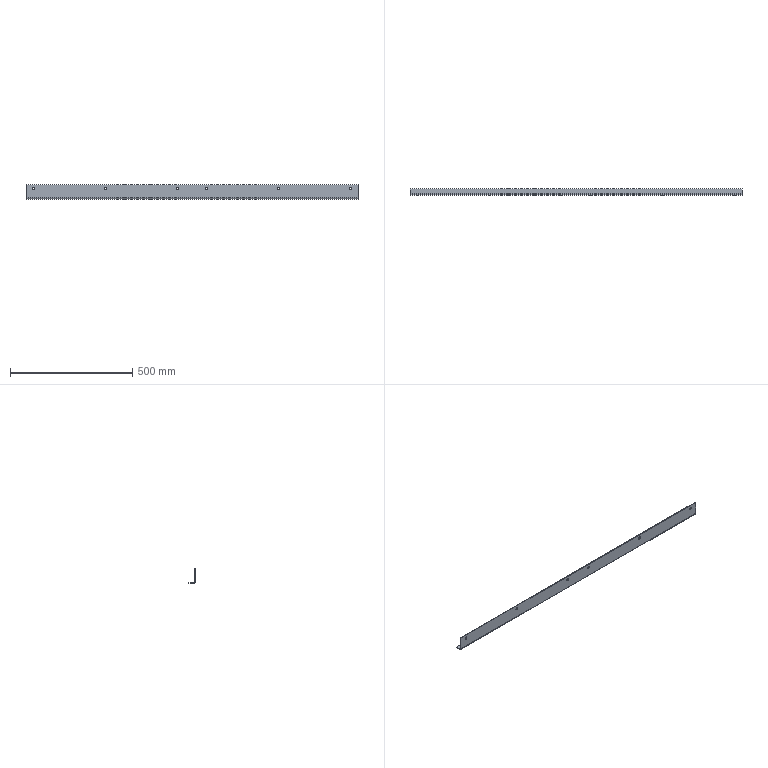Part | STEP file | VD-SYL0380DJ1006_1_1-10_VD-SYL0 | 1 solid | 22 faces | box 1360 x 25 x 60 mm | volume 325121 mm3 | cylinder 14 | plane 8 | commonest cylinder face diameters 10.5 x12 6 x1 12 x1
STEP:
#1=CARTESIAN_POINT('',(-60.,-9.5,39.75));
#2=VERTEX_POINT('',#1);
#3=CARTESIAN_POINT('',(-60.,-9.5,50.25));
#4=VERTEX_POINT('',#3);
#5=CARTESIAN_POINT('',(-60.,-9.5,45.));
#6=DIRECTION('',(0.,-1.,0.));
#7=DIRECTION('',(0.,0.,-1.));
#8=AXIS2_PLACEMENT_3D('',#5,#6,#7);
#9=CIRCLE('',#8,5.25);
#10=EDGE_CURVE('',#2,#4,#9,.T.);
#11=ORIENTED_EDGE('',*,*,#10,.F.);
#12=CARTESIAN_POINT('',(-60.,-12.5,39.75));
#13=VERTEX_POINT('',#12);
#14=CARTESIAN_POINT('',(-60.,-12.5,39.75));
#15=DIRECTION('',(0.,1.,0.));
#16=VECTOR('',#15,1000.);
#17=LINE('',#14,#16);
#18=EDGE_CURVE('',#13,#2,#17,.T.);
#19=ORIENTED_EDGE('',*,*,#18,.F.);
#20=CARTESIAN_POINT('',(-60.,-12.5,50.25));
#21=VERTEX_POINT('',#20);
#22=CARTESIAN_POINT('',(-60.,-12.5,45.));
#23=DIRECTION('',(0.,1.,0.));
#24=DIRECTION('',(0.,0.,1.));
#25=AXIS2_PLACEMENT_3D('',#22,#23,#24);
#26=CIRCLE('',#25,5.25);
#27=EDGE_CURVE('',#21,#13,#26,.T.);
#28=ORIENTED_EDGE('',*,*,#27,.F.);
#29=CARTESIAN_POINT('',(-60.,-12.5,50.25));
#30=DIRECTION('',(0.,1.,0.));
#31=VECTOR('',#30,1000.);
#32=LINE('',#29,#31);
#33=EDGE_CURVE('',#21,#4,#32,.T.);
#34=ORIENTED_EDGE('',*,*,#33,.T.);
#35=EDGE_LOOP('',(#11,#19,#28,#34));
#36=FACE_OUTER_BOUND('',#35,.T.);
#37=CARTESIAN_POINT('',(-60.,-11.,45.));
#38=DIRECTION('',(0.,-1.,0.));
#39=DIRECTION('',(0.,0.,-1.));
#40=AXIS2_PLACEMENT_3D('',#37,#38,#39);
#41=CYLINDRICAL_SURFACE('',#40,5.25);
#42=ADVANCED_FACE('',(#36),#41,.F.);
#43=ORIENTED_EDGE('',*,*,#33,.F.);
#44=CARTESIAN_POINT('',(-60.,-12.5,45.));
#45=DIRECTION('',(0.,1.,0.));
#46=DIRECTION('',(0.,0.,-1.));
#47=AXIS2_PLACEMENT_3D('',#44,#45,#46);
#48=CIRCLE('',#47,5.25);
#49=EDGE_CURVE('',#13,#21,#48,.T.);
#50=ORIENTED_EDGE('',*,*,#49,.F.);
#51=ORIENTED_EDGE('',*,*,#18,.T.);
#52=CARTESIAN_POINT('',(-60.,-9.5,45.));
#53=DIRECTION('',(0.,-1.,0.));
#54=DIRECTION('',(0.,0.,1.));
#55=AXIS2_PLACEMENT_3D('',#52,#53,#54);
#56=CIRCLE('',#55,5.25);
#57=EDGE_CURVE('',#4,#2,#56,.T.);
#58=ORIENTED_EDGE('',*,*,#57,.F.);
#59=EDGE_LOOP('',(#43,#50,#51,#58));
#60=FACE_OUTER_BOUND('',#59,.T.);
#61=CARTESIAN_POINT('',(-60.,-11.,45.));
#62=DIRECTION('',(0.,-1.,0.));
#63=DIRECTION('',(0.,0.,-1.));
#64=AXIS2_PLACEMENT_3D('',#61,#62,#63);
#65=CYLINDRICAL_SURFACE('',#64,5.25);
#66=ADVANCED_FACE('',(#60),#65,.F.);
#67=CARTESIAN_POINT('',(-355.,-9.5,39.75));
#68=VERTEX_POINT('',#67);
#69=CARTESIAN_POINT('',(-355.,-9.5,50.25));
#70=VERTEX_POINT('',#69);
#71=CARTESIAN_POINT('',(-355.,-9.5,45.));
#72=DIRECTION('',(0.,-1.,0.));
#73=DIRECTION('',(0.,0.,-1.));
#74=AXIS2_PLACEMENT_3D('',#71,#72,#73);
#75=CIRCLE('',#74,5.25);
#76=EDGE_CURVE('',#68,#70,#75,.T.);
#77=ORIENTED_EDGE('',*,*,#76,.F.);
#78=CARTESIAN_POINT('',(-355.,-12.5,39.75));
#79=VERTEX_POINT('',#78);
#80=CARTESIAN_POINT('',(-355.,-12.5,39.75));
#81=DIRECTION('',(0.,1.,0.));
#82=VECTOR('',#81,1000.);
#83=LINE('',#80,#82);
#84=EDGE_CURVE('',#79,#68,#83,.T.);
#85=ORIENTED_EDGE('',*,*,#84,.F.);
#86=CARTESIAN_POINT('',(-355.,-12.5,50.25));
#87=VERTEX_POINT('',#86);
#88=CARTESIAN_POINT('',(-355.,-12.5,45.));
#89=DIRECTION('',(0.,1.,0.));
#90=DIRECTION('',(0.,0.,1.));
#91=AXIS2_PLACEMENT_3D('',#88,#89,#90);
#92=CIRCLE('',#91,5.25);
#93=EDGE_CURVE('',#87,#79,#92,.T.);
#94=ORIENTED_EDGE('',*,*,#93,.F.);
#95=CARTESIAN_POINT('',(-355.,-12.5,50.25));
#96=DIRECTION('',(0.,1.,0.));
#97=VECTOR('',#96,1000.);
#98=LINE('',#95,#97);
#99=EDGE_CURVE('',#87,#70,#98,.T.);
#100=ORIENTED_EDGE('',*,*,#99,.T.);
#101=EDGE_LOOP('',(#77,#85,#94,#100));
#102=FACE_OUTER_BOUND('',#101,.T.);
#103=CARTESIAN_POINT('',(-355.,-11.,45.));
#104=DIRECTION('',(0.,-1.,0.));
#105=DIRECTION('',(0.,0.,-1.));
#106=AXIS2_PLACEMENT_3D('',#103,#104,#105);
#107=CYLINDRICAL_SURFACE('',#106,5.25);
#108=ADVANCED_FACE('',(#102),#107,.F.);
#109=ORIENTED_EDGE('',*,*,#99,.F.);
#110=CARTESIAN_POINT('',(-355.,-12.5,45.));
#111=DIRECTION('',(0.,1.,0.));
#112=DIRECTION('',(0.,0.,-1.));
#113=AXIS2_PLACEMENT_3D('',#110,#111,#112);
#114=CIRCLE('',#113,5.25);
#115=EDGE_CURVE('',#79,#87,#114,.T.);
#116=ORIENTED_EDGE('',*,*,#115,.F.);
#117=ORIENTED_EDGE('',*,*,#84,.T.);
#118=CARTESIAN_POINT('',(-355.,-9.5,45.));
#119=DIRECTION('',(0.,-1.,0.));
#120=DIRECTION('',(0.,0.,1.));
#121=AXIS2_PLACEMENT_3D('',#118,#119,#120);
#122=CIRCLE('',#121,5.25);
#123=EDGE_CURVE('',#70,#68,#122,.T.);
#124=ORIENTED_EDGE('',*,*,#123,.F.);
#125=EDGE_LOOP('',(#109,#116,#117,#124));
#126=FACE_OUTER_BOUND('',#125,.T.);
#127=CARTESIAN_POINT('',(-355.,-11.,45.));
#128=DIRECTION('',(0.,-1.,0.));
#129=DIRECTION('',(0.,0.,-1.));
#130=AXIS2_PLACEMENT_3D('',#127,#128,#129);
#131=CYLINDRICAL_SURFACE('',#130,5.25);
#132=ADVANCED_FACE('',(#126),#131,.F.);
#133=CARTESIAN_POINT('',(-650.,-9.5,39.75));
#134=VERTEX_POINT('',#133);
#135=CARTESIAN_POINT('',(-650.,-9.5,50.25));
#136=VERTEX_POINT('',#135);
#137=CARTESIAN_POINT('',(-650.,-9.5,45.));
#138=DIRECTION('',(0.,-1.,0.));
#139=DIRECTION('',(0.,0.,-1.));
#140=AXIS2_PLACEMENT_3D('',#137,#138,#139);
#141=CIRCLE('',#140,5.25);
#142=EDGE_CURVE('',#134,#136,#141,.T.);
#143=ORIENTED_EDGE('',*,*,#142,.F.);
#144=CARTESIAN_POINT('',(-650.,-12.5,39.75));
#145=VERTEX_POINT('',#144);
#146=CARTESIAN_POINT('',(-650.,-12.5,39.75));
#147=DIRECTION('',(0.,1.,0.));
#148=VECTOR('',#147,1000.);
#149=LINE('',#146,#148);
#150=EDGE_CURVE('',#145,#134,#149,.T.);
#151=ORIENTED_EDGE('',*,*,#150,.F.);
#152=CARTESIAN_POINT('',(-650.,-12.5,50.25));
#153=VERTEX_POINT('',#152);
#154=CARTESIAN_POINT('',(-650.,-12.5,45.));
#155=DIRECTION('',(0.,1.,0.));
#156=DIRECTION('',(0.,0.,1.));
#157=AXIS2_PLACEMENT_3D('',#154,#155,#156);
#158=CIRCLE('',#157,5.25);
#159=EDGE_CURVE('',#153,#145,#158,.T.);
#160=ORIENTED_EDGE('',*,*,#159,.F.);
#161=CARTESIAN_POINT('',(-650.,-12.5,50.25));
#162=DIRECTION('',(0.,1.,0.));
#163=VECTOR('',#162,1000.);
#164=LINE('',#161,#163);
#165=EDGE_CURVE('',#153,#136,#164,.T.);
#166=ORIENTED_EDGE('',*,*,#165,.T.);
#167=EDGE_LOOP('',(#143,#151,#160,#166));
#168=FACE_OUTER_BOUND('',#167,.T.);
#169=CARTESIAN_POINT('',(-650.,-11.,45.));
#170=DIRECTION('',(0.,-1.,0.));
#171=DIRECTION('',(0.,0.,-1.));
#172=AXIS2_PLACEMENT_3D('',#169,#170,#171);
#173=CYLINDRICAL_SURFACE('',#172,5.25);
#174=ADVANCED_FACE('',(#168),#173,.F.);
#175=ORIENTED_EDGE('',*,*,#165,.F.);
#176=CARTESIAN_POINT('',(-650.,-12.5,45.));
#177=DIRECTION('',(0.,1.,0.));
#178=DIRECTION('',(0.,0.,-1.));
#179=AXIS2_PLACEMENT_3D('',#176,#177,#178);
#180=CIRCLE('',#179,5.25);
#181=EDGE_CURVE('',#145,#153,#180,.T.);
#182=ORIENTED_EDGE('',*,*,#181,.F.);
#183=ORIENTED_EDGE('',*,*,#150,.T.);
#184=CARTESIAN_POINT('',(-650.,-9.5,45.));
#185=DIRECTION('',(0.,-1.,0.));
#186=DIRECTION('',(0.,0.,1.));
#187=AXIS2_PLACEMENT_3D('',#184,#185,#186);
#188=CIRCLE('',#187,5.25);
#189=EDGE_CURVE('',#136,#134,#188,.T.);
#190=ORIENTED_EDGE('',*,*,#189,.F.);
#191=EDGE_LOOP('',(#175,#182,#183,#190));
#192=FACE_OUTER_BOUND('',#191,.T.);
#193=CARTESIAN_POINT('',(-650.,-11.,45.));
#194=DIRECTION('',(0.,-1.,0.));
#195=DIRECTION('',(0.,0.,-1.));
#196=AXIS2_PLACEMENT_3D('',#193,#194,#195);
#197=CYLINDRICAL_SURFACE('',#196,5.25);
#198=ADVANCED_FACE('',(#192),#197,.F.);
#199=CARTESIAN_POINT('',(60.,-9.5,39.75));
#200=VERTEX_POINT('',#199);
#201=CARTESIAN_POINT('',(60.,-12.5,39.75));
#202=VERTEX_POINT('',#201);
#203=CARTESIAN_POINT('',(60.,-9.5,39.75));
#204=DIRECTION('',(0.,-1.,0.));
#205=VECTOR('',#204,1000.);
#206=LINE('',#203,#205);
#207=EDGE_CURVE('',#200,#202,#206,.T.);
#208=ORIENTED_EDGE('',*,*,#207,.F.);
#209=CARTESIAN_POINT('',(60.,-9.5,50.25));
#210=VERTEX_POINT('',#209);
#211=CARTESIAN_POINT('',(60.,-9.5,45.));
#212=DIRECTION('',(0.,-1.,0.));
#213=DIRECTION('',(0.,0.,1.));
#214=AXIS2_PLACEMENT_3D('',#211,#212,#213);
#215=CIRCLE('',#214,5.25);
#216=EDGE_CURVE('',#210,#200,#215,.T.);
#217=ORIENTED_EDGE('',*,*,#216,.F.);
#218=CARTESIAN_POINT('',(60.,-12.5,50.25));
#219=VERTEX_POINT('',#218);
#220=CARTESIAN_POINT('',(60.,-9.5,50.25));
#221=DIRECTION('',(0.,-1.,0.));
#222=VECTOR('',#221,1000.);
#223=LINE('',#220,#222);
#224=EDGE_CURVE('',#210,#219,#223,.T.);
#225=ORIENTED_EDGE('',*,*,#224,.T.);
#226=CARTESIAN_POINT('',(60.,-12.5,45.));
#227=DIRECTION('',(0.,1.,0.));
#228=DIRECTION('',(0.,0.,-1.));
#229=AXIS2_PLACEMENT_3D('',#226,#227,#228);
#230=CIRCLE('',#229,5.25);
#231=EDGE_CURVE('',#202,#219,#230,.T.);
#232=ORIENTED_EDGE('',*,*,#231,.F.);
#233=EDGE_LOOP('',(#208,#217,#225,#232));
#234=FACE_OUTER_BOUND('',#233,.T.);
#235=CARTESIAN_POINT('',(60.,-11.,45.));
#236=DIRECTION('',(0.,1.,0.));
#237=DIRECTION('',(0.,0.,1.));
#238=AXIS2_PLACEMENT_3D('',#235,#236,#237);
#239=CYLINDRICAL_SURFACE('',#238,5.25);
#240=ADVANCED_FACE('',(#234),#239,.F.);
#241=CARTESIAN_POINT('',(60.,-12.5,45.));
#242=DIRECTION('',(0.,1.,0.));
#243=DIRECTION('',(0.,0.,1.));
#244=AXIS2_PLACEMENT_3D('',#241,#242,#243);
#245=CIRCLE('',#244,5.25);
#246=EDGE_CURVE('',#219,#202,#245,.T.);
#247=ORIENTED_EDGE('',*,*,#246,.F.);
#248=ORIENTED_EDGE('',*,*,#224,.F.);
#249=CARTESIAN_POINT('',(60.,-9.5,45.));
#250=DIRECTION('',(0.,-1.,0.));
#251=DIRECTION('',(0.,0.,-1.));
#252=AXIS2_PLACEMENT_3D('',#249,#250,#251);
#253=CIRCLE('',#252,5.25);
#254=EDGE_CURVE('',#200,#210,#253,.T.);
#255=ORIENTED_EDGE('',*,*,#254,.F.);
#256=ORIENTED_EDGE('',*,*,#207,.T.);
#257=EDGE_LOOP('',(#247,#248,#255,#256));
#258=FACE_OUTER_BOUND('',#257,.T.);
#259=CARTESIAN_POINT('',(60.,-11.,45.));
#260=DIRECTION('',(0.,1.,0.));
#261=DIRECTION('',(0.,0.,1.));
#262=AXIS2_PLACEMENT_3D('',#259,#260,#261);
#263=CYLINDRICAL_SURFACE('',#262,5.25);
#264=ADVANCED_FACE('',(#258),#263,.F.);
#265=CARTESIAN_POINT('',(355.,-9.5,39.75));
#266=VERTEX_POINT('',#265);
#267=CARTESIAN_POINT('',(355.,-12.5,39.75));
#268=VERTEX_POINT('',#267);
#269=CARTESIAN_POINT('',(355.,-9.5,39.75));
#270=DIRECTION('',(0.,-1.,0.));
#271=VECTOR('',#270,1000.);
#272=LINE('',#269,#271);
#273=EDGE_CURVE('',#266,#268,#272,.T.);
#274=ORIENTED_EDGE('',*,*,#273,.F.);
#275=CARTESIAN_POINT('',(355.,-9.5,50.25));
#276=VERTEX_POINT('',#275);
#277=CARTESIAN_POINT('',(355.,-9.5,45.));
#278=DIRECTION('',(0.,-1.,0.));
#279=DIRECTION('',(0.,0.,1.));
#280=AXIS2_PLACEMENT_3D('',#277,#278,#279);
#281=CIRCLE('',#280,5.25);
#282=EDGE_CURVE('',#276,#266,#281,.T.);
#283=ORIENTED_EDGE('',*,*,#282,.F.);
#284=CARTESIAN_POINT('',(355.,-12.5,50.25));
#285=VERTEX_POINT('',#284);
#286=CARTESIAN_POINT('',(355.,-9.5,50.25));
#287=DIRECTION('',(0.,-1.,0.));
#288=VECTOR('',#287,1000.);
#289=LINE('',#286,#288);
#290=EDGE_CURVE('',#276,#285,#289,.T.);
#291=ORIENTED_EDGE('',*,*,#290,.T.);
#292=CARTESIAN_POINT('',(355.,-12.5,45.));
#293=DIRECTION('',(0.,1.,0.));
#294=DIRECTION('',(0.,0.,-1.));
#295=AXIS2_PLACEMENT_3D('',#292,#293,#294);
#296=CIRCLE('',#295,5.25);
#297=EDGE_CURVE('',#268,#285,#296,.T.);
#298=ORIENTED_EDGE('',*,*,#297,.F.);
#299=EDGE_LOOP('',(#274,#283,#291,#298));
#300=FACE_OUTER_BOUND('',#299,.T.);
#301=CARTESIAN_POINT('',(355.,-11.,45.));
#302=DIRECTION('',(0.,1.,0.));
#303=DIRECTION('',(0.,0.,1.));
#304=AXIS2_PLACEMENT_3D('',#301,#302,#303);
#305=CYLINDRICAL_SURFACE('',#304,5.25);
#306=ADVANCED_FACE('',(#300),#305,.F.);
#307=CARTESIAN_POINT('',(355.,-12.5,45.));
#308=DIRECTION('',(0.,1.,0.));
#309=DIRECTION('',(0.,0.,1.));
#310=AXIS2_PLACEMENT_3D('',#307,#308,#309);
#311=CIRCLE('',#310,5.25);
#312=EDGE_CURVE('',#285,#268,#311,.T.);
#313=ORIENTED_EDGE('',*,*,#312,.F.);
#314=ORIENTED_EDGE('',*,*,#290,.F.);
#315=CARTESIAN_POINT('',(355.,-9.5,45.));
#316=DIRECTION('',(0.,-1.,0.));
#317=DIRECTION('',(0.,0.,-1.));
#318=AXIS2_PLACEMENT_3D('',#315,#316,#317);
#319=CIRCLE('',#318,5.25);
#320=EDGE_CURVE('',#266,#276,#319,.T.);
#321=ORIENTED_EDGE('',*,*,#320,.F.);
#322=ORIENTED_EDGE('',*,*,#273,.T.);
#323=EDGE_LOOP('',(#313,#314,#321,#322));
#324=FACE_OUTER_BOUND('',#323,.T.);
#325=CARTESIAN_POINT('',(355.,-11.,45.));
#326=DIRECTION('',(0.,1.,0.));
#327=DIRECTION('',(0.,0.,1.));
#328=AXIS2_PLACEMENT_3D('',#325,#326,#327);
#329=CYLINDRICAL_SURFACE('',#328,5.25);
#330=ADVANCED_FACE('',(#324),#329,.F.);
#331=CARTESIAN_POINT('',(650.,-9.5,39.75));
#332=VERTEX_POINT('',#331);
#333=CARTESIAN_POINT('',(650.,-12.5,39.75));
#334=VERTEX_POINT('',#333);
#335=CARTESIAN_POINT('',(650.,-9.5,39.75));
#336=DIRECTION('',(0.,-1.,0.));
#337=VECTOR('',#336,1000.);
#338=LINE('',#335,#337);
#339=EDGE_CURVE('',#332,#334,#338,.T.);
#340=ORIENTED_EDGE('',*,*,#339,.F.);
#341=CARTESIAN_POINT('',(650.,-9.5,50.25));
#342=VERTEX_POINT('',#341);
#343=CARTESIAN_POINT('',(650.,-9.5,45.));
#344=DIRECTION('',(0.,-1.,0.));
#345=DIRECTION('',(0.,0.,1.));
#346=AXIS2_PLACEMENT_3D('',#343,#344,#345);
#347=CIRCLE('',#346,5.25);
#348=EDGE_CURVE('',#342,#332,#347,.T.);
#349=ORIENTED_EDGE('',*,*,#348,.F.);
#350=CARTESIAN_POINT('',(650.,-12.5,50.25));
#351=VERTEX_POINT('',#350);
#352=CARTESIAN_POINT('',(650.,-9.5,50.25));
#353=DIRECTION('',(0.,-1.,0.));
#354=VECTOR('',#353,1000.);
#355=LINE('',#352,#354);
#356=EDGE_CURVE('',#342,#351,#355,.T.);
#357=ORIENTED_EDGE('',*,*,#356,.T.);
#358=CARTESIAN_POINT('',(650.,-12.5,45.));
#359=DIRECTION('',(0.,1.,0.));
#360=DIRECTION('',(0.,0.,-1.));
#361=AXIS2_PLACEMENT_3D('',#358,#359,#360);
#362=CIRCLE('',#361,5.25);
#363=EDGE_CURVE('',#334,#351,#362,.T.);
#364=ORIENTED_EDGE('',*,*,#363,.F.);
#365=EDGE_LOOP('',(#340,#349,#357,#364));
#366=FACE_OUTER_BOUND('',#365,.T.);
#367=CARTESIAN_POINT('',(650.,-11.,45.));
#368=DIRECTION('',(0.,1.,0.));
#369=DIRECTION('',(0.,0.,1.));
#370=AXIS2_PLACEMENT_3D('',#367,#368,#369);
#371=CYLINDRICAL_SURFACE('',#370,5.25);
#372=ADVANCED_FACE('',(#366),#371,.F.);
#373=CARTESIAN_POINT('',(650.,-12.5,45.));
#374=DIRECTION('',(0.,1.,0.));
#375=DIRECTION('',(0.,0.,1.));
#376=AXIS2_PLACEMENT_3D('',#373,#374,#375);
#377=CIRCLE('',#376,5.25);
#378=EDGE_CURVE('',#351,#334,#377,.T.);
#379=ORIENTED_EDGE('',*,*,#378,.F.);
#380=ORIENTED_EDGE('',*,*,#356,.F.);
#381=CARTESIAN_POINT('',(650.,-9.5,45.));
#382=DIRECTION('',(0.,-1.,0.));
#383=DIRECTION('',(0.,0.,-1.));
#384=AXIS2_PLACEMENT_3D('',#381,#382,#383);
#385=CIRCLE('',#384,5.25);
#386=EDGE_CURVE('',#332,#342,#385,.T.);
#387=ORIENTED_EDGE('',*,*,#386,.F.);
#388=ORIENTED_EDGE('',*,*,#339,.T.);
#389=EDGE_LOOP('',(#379,#380,#387,#388));
#390=FACE_OUTER_BOUND('',#389,.T.);
#391=CARTESIAN_POINT('',(650.,-11.,45.));
#392=DIRECTION('',(0.,1.,0.));
#393=DIRECTION('',(0.,0.,1.));
#394=AXIS2_PLACEMENT_3D('',#391,#392,#393);
#395=CYLINDRICAL_SURFACE('',#394,5.25);
#396=ADVANCED_FACE('',(#390),#395,.F.);
#397=CARTESIAN_POINT('',(-680.,-6.5,0.));
#398=VERTEX_POINT('',#397);
#399=CARTESIAN_POINT('',(680.,-6.5,0.));
#400=VERTEX_POINT('',#399);
#401=CARTESIAN_POINT('',(-680.,-6.5,0.));
#402=DIRECTION('',(1.,0.,0.));
#403=VECTOR('',#402,1000.);
#404=LINE('',#401,#403);
#405=EDGE_CURVE('',#398,#400,#404,.T.);
#406=ORIENTED_EDGE('',*,*,#405,.F.);
#407=CARTESIAN_POINT('',(-680.,12.5,0.));
#408=VERTEX_POINT('',#407);
#409=CARTESIAN_POINT('',(-680.,-6.5,0.));
#410=DIRECTION('',(0.,1.,0.));
#411=VECTOR('',#410,1000.);
#412=LINE('',#409,#411);
#413=EDGE_CURVE('',#398,#408,#412,.T.);
#414=ORIENTED_EDGE('',*,*,#413,.T.);
#415=CARTESIAN_POINT('',(680.,12.5,0.));
#416=VERTEX_POINT('',#415);
#417=CARTESIAN_POINT('',(-680.,12.5,0.));
#418=DIRECTION('',(1.,0.,0.));
#419=VECTOR('',#418,1000.);
#420=LINE('',#417,#419);
#421=EDGE_CURVE('',#408,#416,#420,.T.);
#422=ORIENTED_EDGE('',*,*,#421,.T.);
#423=CARTESIAN_POINT('',(680.,12.5,0.));
#424=DIRECTION('',(0.,-1.,0.));
#425=VECTOR('',#424,1000.);
#426=LINE('',#423,#425);
#427=EDGE_CURVE('',#416,#400,#426,.T.);
#428=ORIENTED_EDGE('',*,*,#427,.T.);
#429=EDGE_LOOP('',(#406,#414,#422,#428));
#430=FACE_OUTER_BOUND('',#429,.T.);
#431=CARTESIAN_POINT('',(0.,0.,0.));
#432=DIRECTION('',(0.,0.,1.));
#433=DIRECTION('',(1.,0.,0.));
#434=AXIS2_PLACEMENT_3D('',#431,#432,#433);
#435=PLANE('',#434);
#436=ADVANCED_FACE('',(#430),#435,.F.);
#437=CARTESIAN_POINT('',(680.,-12.5,6.));
#438=VERTEX_POINT('',#437);
#439=CARTESIAN_POINT('',(-680.,-12.5,6.));
#440=VERTEX_POINT('',#439);
#441=CARTESIAN_POINT('',(680.,-12.5,6.));
#442=DIRECTION('',(-1.,0.,0.));
#443=VECTOR('',#442,1000.);
#444=LINE('',#441,#443);
#445=EDGE_CURVE('',#438,#440,#444,.T.);
#446=ORIENTED_EDGE('',*,*,#445,.T.);
#447=CARTESIAN_POINT('',(-680.,-6.5,6.));
#448=DIRECTION('',(-1.,0.,0.));
#449=DIRECTION('',(0.,0.,-1.));
#450=AXIS2_PLACEMENT_3D('',#447,#448,#449);
#451=CIRCLE('',#450,6.);
#452=EDGE_CURVE('',#398,#440,#451,.T.);
#453=ORIENTED_EDGE('',*,*,#452,.F.);
#454=ORIENTED_EDGE('',*,*,#405,.T.);
#455=CARTESIAN_POINT('',(680.,-6.5,6.));
#456=DIRECTION('',(1.,0.,0.));
#457=DIRECTION('',(0.,-1.,0.));
#458=AXIS2_PLACEMENT_3D('',#455,#456,#457);
#459=CIRCLE('',#458,6.);
#460=EDGE_CURVE('',#438,#400,#459,.T.);
#461=ORIENTED_EDGE('',*,*,#460,.F.);
#462=EDGE_LOOP('',(#446,#453,#454,#461));
#463=FACE_OUTER_BOUND('',#462,.T.);
#464=CARTESIAN_POINT('',(-680.,-6.5,6.));
#465=DIRECTION('',(1.,0.,0.));
#466=DIRECTION('',(0.,0.,-1.));
#467=AXIS2_PLACEMENT_3D('',#464,#465,#466);
#468=CYLINDRICAL_SURFACE('',#467,6.);
#469=ADVANCED_FACE('',(#463),#468,.T.);
#470=ORIENTED_EDGE('',*,*,#27,.T.);
#471=ORIENTED_EDGE('',*,*,#49,.T.);
#472=EDGE_LOOP('',(#470,#471));
#473=FACE_BOUND('',#472,.T.);
#474=ORIENTED_EDGE('',*,*,#93,.T.);
#475=ORIENTED_EDGE('',*,*,#115,.T.);
#476=EDGE_LOOP('',(#474,#475));
#477=FACE_BOUND('',#476,.T.);
#478=ORIENTED_EDGE('',*,*,#159,.T.);
#479=ORIENTED_EDGE('',*,*,#181,.T.);
#480=EDGE_LOOP('',(#478,#479));
#481=FACE_BOUND('',#480,.T.);
#482=ORIENTED_EDGE('',*,*,#231,.T.);
#483=ORIENTED_EDGE('',*,*,#246,.T.);
#484=EDGE_LOOP('',(#482,#483));
#485=FACE_BOUND('',#484,.T.);
#486=ORIENTED_EDGE('',*,*,#297,.T.);
#487=ORIENTED_EDGE('',*,*,#312,.T.);
#488=EDGE_LOOP('',(#486,#487));
#489=FACE_BOUND('',#488,.T.);
#490=ORIENTED_EDGE('',*,*,#363,.T.);
#491=ORIENTED_EDGE('',*,*,#378,.T.);
#492=EDGE_LOOP('',(#490,#491));
#493=FACE_BOUND('',#492,.T.);
#494=CARTESIAN_POINT('',(680.,-12.5,60.));
#495=VERTEX_POINT('',#494);
#496=CARTESIAN_POINT('',(680.,-12.5,60.));
#497=DIRECTION('',(0.,0.,-1.));
#498=VECTOR('',#497,1000.);
#499=LINE('',#496,#498);
#500=EDGE_CURVE('',#495,#438,#499,.T.);
#501=ORIENTED_EDGE('',*,*,#500,.F.);
#502=CARTESIAN_POINT('',(-680.,-12.5,60.));
#503=VERTEX_POINT('',#502);
#504=CARTESIAN_POINT('',(-680.,-12.5,60.));
#505=DIRECTION('',(1.,0.,0.));
#506=VECTOR('',#505,1000.);
#507=LINE('',#504,#506);
#508=EDGE_CURVE('',#503,#495,#507,.T.);
#509=ORIENTED_EDGE('',*,*,#508,.F.);
#510=CARTESIAN_POINT('',(-680.,-12.5,6.));
#511=DIRECTION('',(0.,0.,1.));
#512=VECTOR('',#511,1000.);
#513=LINE('',#510,#512);
#514=EDGE_CURVE('',#440,#503,#513,.T.);
#515=ORIENTED_EDGE('',*,*,#514,.F.);
#516=ORIENTED_EDGE('',*,*,#445,.F.);
#517=EDGE_LOOP('',(#501,#509,#515,#516));
#518=FACE_OUTER_BOUND('',#517,.T.);
#519=CARTESIAN_POINT('',(680.,-12.5,0.));
#520=DIRECTION('',(0.,-1.,0.));
#521=DIRECTION('',(0.,0.,-1.));
#522=AXIS2_PLACEMENT_3D('',#519,#520,#521);
#523=PLANE('',#522);
#524=ADVANCED_FACE('',(#473,#477,#481,#485,#489,#493,#518),#523,.T.);
#525=ORIENTED_EDGE('',*,*,#508,.T.);
#526=CARTESIAN_POINT('',(680.,-9.5,60.));
#527=VERTEX_POINT('',#526);
#528=CARTESIAN_POINT('',(680.,-12.5,60.));
#529=DIRECTION('',(0.,1.,0.));
#530=VECTOR('',#529,1000.);
#531=LINE('',#528,#530);
#532=EDGE_CURVE('',#495,#527,#531,.T.);
#533=ORIENTED_EDGE('',*,*,#532,.T.);
#534=CARTESIAN_POINT('',(-680.,-9.5,60.));
#535=VERTEX_POINT('',#534);
#536=CARTESIAN_POINT('',(-680.,-9.5,60.));
#537=DIRECTION('',(1.,0.,0.));
#538=VECTOR('',#537,1000.);
#539=LINE('',#536,#538);
#540=EDGE_CURVE('',#535,#527,#539,.T.);
#541=ORIENTED_EDGE('',*,*,#540,.F.);
#542=CARTESIAN_POINT('',(-680.,-9.5,60.));
#543=DIRECTION('',(0.,-1.,0.));
#544=VECTOR('',#543,1000.);
#545=LINE('',#542,#544);
#546=EDGE_CURVE('',#535,#503,#545,.T.);
#547=ORIENTED_EDGE('',*,*,#546,.T.);
#548=EDGE_LOOP('',(#525,#533,#541,#547));
#549=FACE_OUTER_BOUND('',#548,.T.);
#550=CARTESIAN_POINT('',(0.,-11.,60.));
#551=DIRECTION('',(0.,0.,1.));
#552=DIRECTION('',(1.,0.,0.));
#553=AXIS2_PLACEMENT_3D('',#550,#551,#552);
#554=PLANE('',#553);
#555=ADVANCED_FACE('',(#549),#554,.T.);
#556=ORIENTED_EDGE('',*,*,#500,.T.);
#557=ORIENTED_EDGE('',*,*,#460,.T.);
#558=ORIENTED_EDGE('',*,*,#427,.F.);
#559=CARTESIAN_POINT('',(680.,12.5,3.));
#560=VERTEX_POINT('',#559);
#561=CARTESIAN_POINT('',(680.,12.5,0.));
#562=DIRECTION('',(0.,0.,1.));
#563=VECTOR('',#562,1000.);
#564=LINE('',#561,#563);
#565=EDGE_CURVE('',#416,#560,#564,.T.);
#566=ORIENTED_EDGE('',*,*,#565,.T.);
#567=CARTESIAN_POINT('',(680.,-6.5,3.));
#568=VERTEX_POINT('',#567);
#569=CARTESIAN_POINT('',(680.,12.5,3.));
#570=DIRECTION('',(0.,-1.,0.));
#571=VECTOR('',#570,1000.);
#572=LINE('',#569,#571);
#573=EDGE_CURVE('',#560,#568,#572,.T.);
#574=ORIENTED_EDGE('',*,*,#573,.T.);
#575=CARTESIAN_POINT('',(680.,-9.5,6.));
#576=VERTEX_POINT('',#575);
#577=CARTESIAN_POINT('',(680.,-6.5,6.));
#578=DIRECTION('',(-1.,0.,0.));
#579=DIRECTION('',(0.,0.,-1.));
#580=AXIS2_PLACEMENT_3D('',#577,#578,#579);
#581=CIRCLE('',#580,3.);
#582=EDGE_CURVE('',#568,#576,#581,.T.);
#583=ORIENTED_EDGE('',*,*,#582,.T.);
#584=CARTESIAN_POINT('',(680.,-9.5,60.));
#585=DIRECTION('',(0.,0.,-1.));
#586=VECTOR('',#585,1000.);
#587=LINE('',#584,#586);
#588=EDGE_CURVE('',#527,#576,#587,.T.);
#589=ORIENTED_EDGE('',*,*,#588,.F.);
#590=ORIENTED_EDGE('',*,*,#532,.F.);
#591=EDGE_LOOP('',(#556,#557,#558,#566,#574,#583,#589,#590));
#592=FACE_OUTER_BOUND('',#591,.T.);
#593=CARTESIAN_POINT('',(680.,-11.,33.));
#594=DIRECTION('',(1.,0.,0.));
#595=DIRECTION('',(0.,1.,0.));
#596=AXIS2_PLACEMENT_3D('',#593,#594,#595);
#597=PLANE('',#596);
#598=ADVANCED_FACE('',(#592),#597,.T.);
#599=ORIENTED_EDGE('',*,*,#57,.T.);
#600=ORIENTED_EDGE('',*,*,#10,.T.);
#601=EDGE_LOOP('',(#599,#600));
#602=FACE_BOUND('',#601,.T.);
#603=ORIENTED_EDGE('',*,*,#123,.T.);
#604=ORIENTED_EDGE('',*,*,#76,.T.);
#605=EDGE_LOOP('',(#603,#604));
#606=FACE_BOUND('',#605,.T.);
#607=ORIENTED_EDGE('',*,*,#189,.T.);
#608=ORIENTED_EDGE('',*,*,#142,.T.);
#609=EDGE_LOOP('',(#607,#608));
#610=FACE_BOUND('',#609,.T.);
#611=ORIENTED_EDGE('',*,*,#254,.T.);
#612=ORIENTED_EDGE('',*,*,#216,.T.);
#613=EDGE_LOOP('',(#611,#612));
#614=FACE_BOUND('',#613,.T.);
#615=ORIENTED_EDGE('',*,*,#320,.T.);
#616=ORIENTED_EDGE('',*,*,#282,.T.);
#617=EDGE_LOOP('',(#615,#616));
#618=FACE_BOUND('',#617,.T.);
#619=ORIENTED_EDGE('',*,*,#386,.T.);
#620=ORIENTED_EDGE('',*,*,#348,.T.);
#621=EDGE_LOOP('',(#619,#620));
#622=FACE_BOUND('',#621,.T.);
#623=ORIENTED_EDGE('',*,*,#540,.T.);
#624=ORIENTED_EDGE('',*,*,#588,.T.);
#625=CARTESIAN_POINT('',(-680.,-9.5,6.));
#626=VERTEX_POINT('',#625);
#627=CARTESIAN_POINT('',(-680.,-9.5,6.));
#628=DIRECTION('',(1.,0.,0.));
#629=VECTOR('',#628,1000.);
#630=LINE('',#627,#629);
#631=EDGE_CURVE('',#626,#576,#630,.T.);
#632=ORIENTED_EDGE('',*,*,#631,.F.);
#633=CARTESIAN_POINT('',(-680.,-9.5,6.));
#634=DIRECTION('',(0.,0.,1.));
#635=VECTOR('',#634,1000.);
#636=LINE('',#633,#635);
#637=EDGE_CURVE('',#626,#535,#636,.T.);
#638=ORIENTED_EDGE('',*,*,#637,.T.);
#639=EDGE_LOOP('',(#623,#624,#632,#638));
#640=FACE_OUTER_BOUND('',#639,.T.);
#641=CARTESIAN_POINT('',(680.,-9.5,0.));
#642=DIRECTION('',(0.,-1.,0.));
#643=DIRECTION('',(0.,0.,-1.));
#644=AXIS2_PLACEMENT_3D('',#641,#642,#643);
#645=PLANE('',#644);
#646=ADVANCED_FACE('',(#602,#606,#610,#614,#618,#622,#640),#645,.F.);
#647=CARTESIAN_POINT('',(-680.,-6.5,3.));
#648=VERTEX_POINT('',#647);
#649=CARTESIAN_POINT('',(-680.,-6.5,6.));
#650=DIRECTION('',(1.,0.,0.));
#651=DIRECTION('',(0.,-1.,0.));
#652=AXIS2_PLACEMENT_3D('',#649,#650,#651);
#653=CIRCLE('',#652,3.);
#654=EDGE_CURVE('',#626,#648,#653,.T.);
#655=ORIENTED_EDGE('',*,*,#654,.T.);
#656=CARTESIAN_POINT('',(-680.,12.5,3.));
#657=VERTEX_POINT('',#656);
#658=CARTESIAN_POINT('',(-680.,-6.5,3.));
#659=DIRECTION('',(0.,1.,0.));
#660=VECTOR('',#659,1000.);
#661=LINE('',#658,#660);
#662=EDGE_CURVE('',#648,#657,#661,.T.);
#663=ORIENTED_EDGE('',*,*,#662,.T.);
#664=CARTESIAN_POINT('',(-680.,12.5,0.));
#665=DIRECTION('',(0.,0.,1.));
#666=VECTOR('',#665,1000.);
#667=LINE('',#664,#666);
#668=EDGE_CURVE('',#408,#657,#667,.T.);
#669=ORIENTED_EDGE('',*,*,#668,.F.);
#670=ORIENTED_EDGE('',*,*,#413,.F.);
#671=ORIENTED_EDGE('',*,*,#452,.T.);
#672=ORIENTED_EDGE('',*,*,#514,.T.);
#673=ORIENTED_EDGE('',*,*,#546,.F.);
#674=ORIENTED_EDGE('',*,*,#637,.F.);
#675=EDGE_LOOP('',(#655,#663,#669,#670,#671,#672,#673,#674));
#676=FACE_OUTER_BOUND('',#675,.T.);
#677=CARTESIAN_POINT('',(-680.,-11.,33.));
#678=DIRECTION('',(-1.,0.,0.));
#679=DIRECTION('',(0.,0.,1.));
#680=AXIS2_PLACEMENT_3D('',#677,#678,#679);
#681=PLANE('',#680);
#682=ADVANCED_FACE('',(#676),#681,.T.);
#683=ORIENTED_EDGE('',*,*,#565,.F.);
#684=ORIENTED_EDGE('',*,*,#421,.F.);
#685=ORIENTED_EDGE('',*,*,#668,.T.);
#686=CARTESIAN_POINT('',(-680.,12.5,3.));
#687=DIRECTION('',(1.,0.,0.));
#688=VECTOR('',#687,1000.);
#689=LINE('',#686,#688);
#690=EDGE_CURVE('',#657,#560,#689,.T.);
#691=ORIENTED_EDGE('',*,*,#690,.T.);
#692=EDGE_LOOP('',(#683,#684,#685,#691));
#693=FACE_OUTER_BOUND('',#692,.T.);
#694=CARTESIAN_POINT('',(0.,12.5,1.5));
#695=DIRECTION('',(0.,-1.,0.));
#696=DIRECTION('',(0.,0.,-1.));
#697=AXIS2_PLACEMENT_3D('',#694,#695,#696);
#698=PLANE('',#697);
#699=ADVANCED_FACE('',(#693),#698,.F.);
#700=ORIENTED_EDGE('',*,*,#662,.F.);
#701=CARTESIAN_POINT('',(680.,-6.5,3.));
#702=DIRECTION('',(-1.,0.,0.));
#703=VECTOR('',#702,1000.);
#704=LINE('',#701,#703);
#705=EDGE_CURVE('',#568,#648,#704,.T.);
#706=ORIENTED_EDGE('',*,*,#705,.F.);
#707=ORIENTED_EDGE('',*,*,#573,.F.);
#708=ORIENTED_EDGE('',*,*,#690,.F.);
#709=EDGE_LOOP('',(#700,#706,#707,#708));
#710=FACE_OUTER_BOUND('',#709,.T.);
#711=CARTESIAN_POINT('',(0.,0.,3.));
#712=DIRECTION('',(0.,0.,1.));
#713=DIRECTION('',(1.,0.,0.));
#714=AXIS2_PLACEMENT_3D('',#711,#712,#713);
#715=PLANE('',#714);
#716=ADVANCED_FACE('',(#710),#715,.T.);
#717=ORIENTED_EDGE('',*,*,#654,.F.);
#718=ORIENTED_EDGE('',*,*,#631,.T.);
#719=ORIENTED_EDGE('',*,*,#582,.F.);
#720=ORIENTED_EDGE('',*,*,#705,.T.);
#721=EDGE_LOOP('',(#717,#718,#719,#720));
#722=FACE_OUTER_BOUND('',#721,.T.);
#723=CARTESIAN_POINT('',(-680.,-6.5,6.));
#724=DIRECTION('',(1.,0.,0.));
#725=DIRECTION('',(0.,0.,-1.));
#726=AXIS2_PLACEMENT_3D('',#723,#724,#725);
#727=CYLINDRICAL_SURFACE('',#726,3.);
#728=ADVANCED_FACE('',(#722),#727,.F.);
#729=CLOSED_SHELL('',(#42,#66,#108,#132,#174,#198,#240,#264,#306,#330,#372,#396,#436,#469,#524,#555,#598,#646,#682,#699,#716,#728));
#730=MANIFOLD_SOLID_BREP('',#729);
#731=CARTESIAN_POINT('',(0.,0.,0.));
#732=DIRECTION('',(0.,0.,1.));
#733=DIRECTION('',(1.,0.,0.));
#734=AXIS2_PLACEMENT_3D('',#731,#732,#733);
#735=(LENGTH_UNIT()NAMED_UNIT(*)SI_UNIT(.MILLI.,.METRE.));
#736=UNCERTAINTY_MEASURE_WITH_UNIT(LENGTH_MEASURE(0.00001),#735,'','');
#737=(NAMED_UNIT(*)PLANE_ANGLE_UNIT()SI_UNIT($,.RADIAN.));
#738=(NAMED_UNIT(*)SI_UNIT($,.STERADIAN.)SOLID_ANGLE_UNIT());
#739=(GEOMETRIC_REPRESENTATION_CONTEXT(3)GLOBAL_UNCERTAINTY_ASSIGNED_CONTEXT((#736))GLOBAL_UNIT_ASSIGNED_CONTEXT((#735,#737,#738))REPRESENTATION_CONTEXT('',''));
#740=ADVANCED_BREP_SHAPE_REPRESENTATION('',(#730,#734),#739);